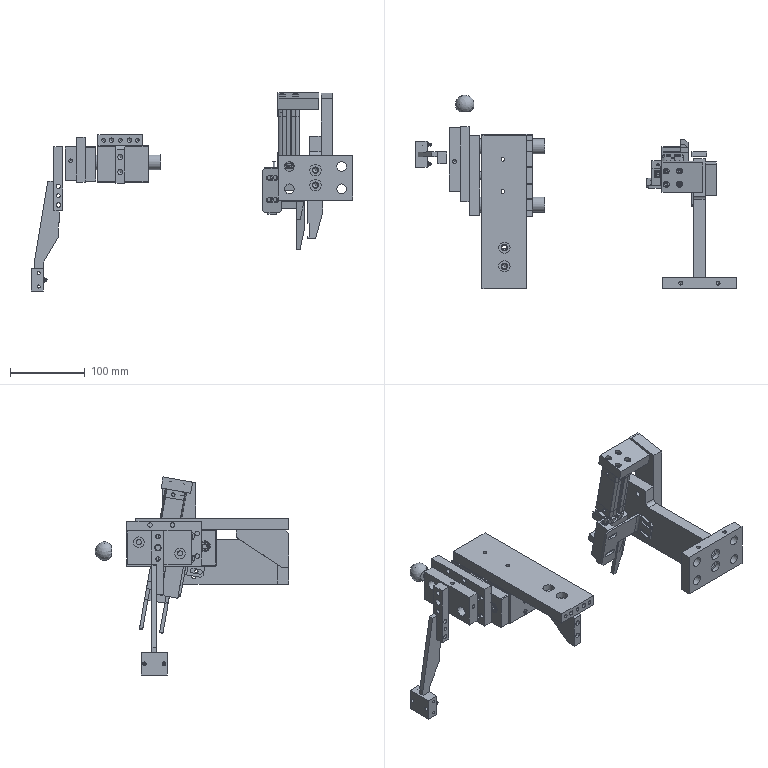Part | NX | features BREP 23 | 26 solids | 1136 faces | box 429.95 x 259 x 264.656 mm | volume 1223129 mm3 | plane 575 | cylinder 430 | cone 121 | torus 5 | sphere 5 | commonest cylinder face diameters 6 x61 0.8 x44 0.4 x32 1.589 x18 2.781 x18 1.2 x16